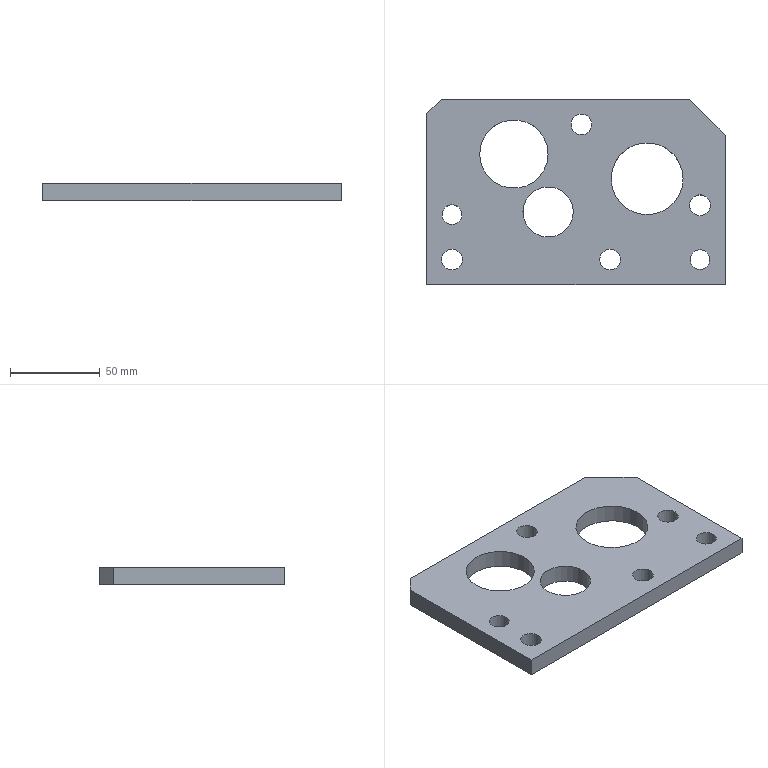Part | STEP file | lll_id4270_x_t | 1 solid | 17 faces | box 166 x 103.25 x 10 mm | volume 132948 mm3 | cylinder 9 | plane 8 | commonest cylinder face diameters 11.509 x4 11 x2 28 x1 38 x1 40 x1
STEP:
#1=CARTESIAN_POINT('',(3399.5,-57.,-45.));
#2=VERTEX_POINT('',#1);
#3=CARTESIAN_POINT('',(3419.5,-57.,-45.));
#4=DIRECTION('',(0.,0.,1.));
#5=DIRECTION('',(-1.,0.,0.));
#6=AXIS2_PLACEMENT_3D('',#3,#4,#5);
#7=CIRCLE('',#6,20.);
#8=EDGE_CURVE('',#2,#2,#7,.T.);
#9=ORIENTED_EDGE('',*,*,#8,.T.);
#10=EDGE_LOOP('',(#9));
#11=FACE_BOUND('',#10,.T.);
#12=CARTESIAN_POINT('',(3443.435,-102.,-45.));
#13=VERTEX_POINT('',#12);
#14=CARTESIAN_POINT('',(3448.935,-102.,-45.));
#15=DIRECTION('',(0.,0.,1.));
#16=DIRECTION('',(-1.,0.,0.));
#17=AXIS2_PLACEMENT_3D('',#14,#15,#16);
#18=CIRCLE('',#17,5.5);
#19=EDGE_CURVE('',#13,#13,#18,.T.);
#20=ORIENTED_EDGE('',*,*,#19,.T.);
#21=EDGE_LOOP('',(#20));
#22=FACE_BOUND('',#21,.T.);
#23=CARTESIAN_POINT('',(3304.935,-12.75,-45.));
#24=VERTEX_POINT('',#23);
#25=CARTESIAN_POINT('',(3442.935,-12.75,-45.));
#26=VERTEX_POINT('',#25);
#27=CARTESIAN_POINT('',(3580.234,-12.75,-45.));
#28=DIRECTION('',(1.,0.,0.));
#29=VECTOR('',#28,1.);
#30=LINE('',#27,#29);
#31=EDGE_CURVE('',#24,#26,#30,.T.);
#32=ORIENTED_EDGE('',*,*,#31,.T.);
#33=CARTESIAN_POINT('',(3462.935,-32.75,-45.));
#34=VERTEX_POINT('',#33);
#35=CARTESIAN_POINT('',(3455.935,-25.75,-45.));
#36=DIRECTION('',(-0.7071,0.7071,0.));
#37=VECTOR('',#36,1.);
#38=LINE('',#35,#37);
#39=EDGE_CURVE('',#34,#26,#38,.T.);
#40=ORIENTED_EDGE('',*,*,#39,.F.);
#41=CARTESIAN_POINT('',(3462.935,-116.,-45.));
#42=VERTEX_POINT('',#41);
#43=CARTESIAN_POINT('',(3462.935,-198.7,-45.));
#44=DIRECTION('',(0.,-1.,0.));
#45=VECTOR('',#44,1.);
#46=LINE('',#43,#45);
#47=EDGE_CURVE('',#34,#42,#46,.T.);
#48=ORIENTED_EDGE('',*,*,#47,.T.);
#49=CARTESIAN_POINT('',(3296.935,-116.,-45.));
#50=VERTEX_POINT('',#49);
#51=CARTESIAN_POINT('',(3580.234,-116.,-45.));
#52=DIRECTION('',(-1.,0.,0.));
#53=VECTOR('',#52,1.);
#54=LINE('',#51,#53);
#55=EDGE_CURVE('',#42,#50,#54,.T.);
#56=ORIENTED_EDGE('',*,*,#55,.T.);
#57=CARTESIAN_POINT('',(3296.935,-20.75,-45.));
#58=VERTEX_POINT('',#57);
#59=CARTESIAN_POINT('',(3296.935,-198.7,-45.));
#60=DIRECTION('',(0.,1.,0.));
#61=VECTOR('',#60,1.);
#62=LINE('',#59,#61);
#63=EDGE_CURVE('',#50,#58,#62,.T.);
#64=ORIENTED_EDGE('',*,*,#63,.T.);
#65=CARTESIAN_POINT('',(3179.435,-138.25,-45.));
#66=DIRECTION('',(-0.7071,-0.7071,0.));
#67=VECTOR('',#66,1.);
#68=LINE('',#65,#67);
#69=EDGE_CURVE('',#24,#58,#68,.T.);
#70=ORIENTED_EDGE('',*,*,#69,.F.);
#71=EDGE_LOOP('',(#32,#40,#48,#56,#64,#70));
#72=FACE_BOUND('',#71,.T.);
#73=CARTESIAN_POINT('',(3305.181,-102.,-45.));
#74=VERTEX_POINT('',#73);
#75=CARTESIAN_POINT('',(3310.935,-102.,-45.));
#76=DIRECTION('',(0.,0.,1.));
#77=DIRECTION('',(-1.,0.,0.));
#78=AXIS2_PLACEMENT_3D('',#75,#76,#77);
#79=CIRCLE('',#78,5.755);
#80=EDGE_CURVE('',#74,#74,#79,.T.);
#81=ORIENTED_EDGE('',*,*,#80,.T.);
#82=EDGE_LOOP('',(#81));
#83=FACE_BOUND('',#82,.T.);
#84=CARTESIAN_POINT('',(3305.435,-77.,-45.));
#85=VERTEX_POINT('',#84);
#86=CARTESIAN_POINT('',(3310.935,-77.,-45.));
#87=DIRECTION('',(0.,0.,1.));
#88=DIRECTION('',(-1.,0.,0.));
#89=AXIS2_PLACEMENT_3D('',#86,#87,#88);
#90=CIRCLE('',#89,5.5);
#91=EDGE_CURVE('',#85,#85,#90,.T.);
#92=ORIENTED_EDGE('',*,*,#91,.T.);
#93=EDGE_LOOP('',(#92));
#94=FACE_BOUND('',#93,.T.);
#95=CARTESIAN_POINT('',(3377.181,-26.75,-45.));
#96=VERTEX_POINT('',#95);
#97=CARTESIAN_POINT('',(3382.935,-26.75,-45.));
#98=DIRECTION('',(0.,0.,1.));
#99=DIRECTION('',(-1.,0.,0.));
#100=AXIS2_PLACEMENT_3D('',#97,#98,#99);
#101=CIRCLE('',#100,5.755);
#102=EDGE_CURVE('',#96,#96,#101,.T.);
#103=ORIENTED_EDGE('',*,*,#102,.T.);
#104=EDGE_LOOP('',(#103));
#105=FACE_BOUND('',#104,.T.);
#106=CARTESIAN_POINT('',(3393.181,-102.,-45.));
#107=VERTEX_POINT('',#106);
#108=CARTESIAN_POINT('',(3398.935,-102.,-45.));
#109=DIRECTION('',(0.,0.,1.));
#110=DIRECTION('',(-1.,0.,0.));
#111=AXIS2_PLACEMENT_3D('',#108,#109,#110);
#112=CIRCLE('',#111,5.755);
#113=EDGE_CURVE('',#107,#107,#112,.T.);
#114=ORIENTED_EDGE('',*,*,#113,.T.);
#115=EDGE_LOOP('',(#114));
#116=FACE_BOUND('',#115,.T.);
#117=CARTESIAN_POINT('',(3443.181,-71.75,-45.));
#118=VERTEX_POINT('',#117);
#119=CARTESIAN_POINT('',(3448.935,-71.75,-45.));
#120=DIRECTION('',(0.,0.,1.));
#121=DIRECTION('',(-1.,0.,0.));
#122=AXIS2_PLACEMENT_3D('',#119,#120,#121);
#123=CIRCLE('',#122,5.755);
#124=EDGE_CURVE('',#118,#118,#123,.T.);
#125=ORIENTED_EDGE('',*,*,#124,.T.);
#126=EDGE_LOOP('',(#125));
#127=FACE_BOUND('',#126,.T.);
#128=CARTESIAN_POINT('',(3350.435,-75.5,-45.));
#129=VERTEX_POINT('',#128);
#130=CARTESIAN_POINT('',(3364.435,-75.5,-45.));
#131=DIRECTION('',(0.,0.,-1.));
#132=DIRECTION('',(-1.,0.,0.));
#133=AXIS2_PLACEMENT_3D('',#130,#131,#132);
#134=CIRCLE('',#133,14.);
#135=EDGE_CURVE('',#129,#129,#134,.T.);
#136=ORIENTED_EDGE('',*,*,#135,.F.);
#137=EDGE_LOOP('',(#136));
#138=FACE_BOUND('',#137,.T.);
#139=CARTESIAN_POINT('',(3326.367,-43.288,-45.));
#140=VERTEX_POINT('',#139);
#141=CARTESIAN_POINT('',(3345.367,-43.288,-45.));
#142=DIRECTION('',(0.,0.,1.));
#143=DIRECTION('',(-1.,0.,0.));
#144=AXIS2_PLACEMENT_3D('',#141,#142,#143);
#145=CIRCLE('',#144,19.);
#146=EDGE_CURVE('',#140,#140,#145,.T.);
#147=ORIENTED_EDGE('',*,*,#146,.T.);
#148=EDGE_LOOP('',(#147));
#149=FACE_BOUND('',#148,.T.);
#150=CARTESIAN_POINT('',(3580.234,-198.7,-45.));
#151=DIRECTION('',(0.,0.,-1.));
#152=DIRECTION('',(0.,-1.,0.));
#153=AXIS2_PLACEMENT_3D('',#150,#151,#152);
#154=PLANE('',#153);
#155=ADVANCED_FACE('',(#11,#22,#72,#83,#94,#105,#116,#127,#138,#149),#154,.T.);
#156=CARTESIAN_POINT('',(3399.5,-57.,-35.));
#157=VERTEX_POINT('',#156);
#158=CARTESIAN_POINT('',(3419.5,-57.,-35.));
#159=DIRECTION('',(0.,0.,1.));
#160=DIRECTION('',(-1.,0.,0.));
#161=AXIS2_PLACEMENT_3D('',#158,#159,#160);
#162=CIRCLE('',#161,20.);
#163=EDGE_CURVE('',#157,#157,#162,.T.);
#164=ORIENTED_EDGE('',*,*,#163,.F.);
#165=EDGE_LOOP('',(#164));
#166=FACE_BOUND('',#165,.T.);
#167=CARTESIAN_POINT('',(3443.435,-102.,-35.));
#168=VERTEX_POINT('',#167);
#169=CARTESIAN_POINT('',(3448.935,-102.,-35.));
#170=DIRECTION('',(0.,0.,1.));
#171=DIRECTION('',(-1.,0.,0.));
#172=AXIS2_PLACEMENT_3D('',#169,#170,#171);
#173=CIRCLE('',#172,5.5);
#174=EDGE_CURVE('',#168,#168,#173,.T.);
#175=ORIENTED_EDGE('',*,*,#174,.F.);
#176=EDGE_LOOP('',(#175));
#177=FACE_BOUND('',#176,.T.);
#178=CARTESIAN_POINT('',(3304.935,-12.75,-35.));
#179=VERTEX_POINT('',#178);
#180=CARTESIAN_POINT('',(3442.935,-12.75,-35.));
#181=VERTEX_POINT('',#180);
#182=CARTESIAN_POINT('',(3266.435,-12.75,-35.));
#183=DIRECTION('',(1.,0.,0.));
#184=VECTOR('',#183,1.);
#185=LINE('',#182,#184);
#186=EDGE_CURVE('',#179,#181,#185,.T.);
#187=ORIENTED_EDGE('',*,*,#186,.F.);
#188=CARTESIAN_POINT('',(3296.935,-20.75,-35.));
#189=VERTEX_POINT('',#188);
#190=CARTESIAN_POINT('',(3179.435,-138.25,-35.));
#191=DIRECTION('',(-0.7071,-0.7071,0.));
#192=VECTOR('',#191,1.);
#193=LINE('',#190,#192);
#194=EDGE_CURVE('',#179,#189,#193,.T.);
#195=ORIENTED_EDGE('',*,*,#194,.T.);
#196=CARTESIAN_POINT('',(3296.935,-116.,-35.));
#197=VERTEX_POINT('',#196);
#198=CARTESIAN_POINT('',(3296.935,-215.25,-35.));
#199=DIRECTION('',(0.,1.,0.));
#200=VECTOR('',#199,1.);
#201=LINE('',#198,#200);
#202=EDGE_CURVE('',#197,#189,#201,.T.);
#203=ORIENTED_EDGE('',*,*,#202,.F.);
#204=CARTESIAN_POINT('',(3462.935,-116.,-35.));
#205=VERTEX_POINT('',#204);
#206=CARTESIAN_POINT('',(3266.435,-116.,-35.));
#207=DIRECTION('',(-1.,0.,0.));
#208=VECTOR('',#207,1.);
#209=LINE('',#206,#208);
#210=EDGE_CURVE('',#205,#197,#209,.T.);
#211=ORIENTED_EDGE('',*,*,#210,.F.);
#212=CARTESIAN_POINT('',(3462.935,-32.75,-35.));
#213=VERTEX_POINT('',#212);
#214=CARTESIAN_POINT('',(3462.935,-215.25,-35.));
#215=DIRECTION('',(0.,-1.,0.));
#216=VECTOR('',#215,1.);
#217=LINE('',#214,#216);
#218=EDGE_CURVE('',#213,#205,#217,.T.);
#219=ORIENTED_EDGE('',*,*,#218,.F.);
#220=CARTESIAN_POINT('',(3455.935,-25.75,-35.));
#221=DIRECTION('',(-0.7071,0.7071,0.));
#222=VECTOR('',#221,1.);
#223=LINE('',#220,#222);
#224=EDGE_CURVE('',#213,#181,#223,.T.);
#225=ORIENTED_EDGE('',*,*,#224,.T.);
#226=EDGE_LOOP('',(#187,#195,#203,#211,#219,#225));
#227=FACE_BOUND('',#226,.T.);
#228=CARTESIAN_POINT('',(3305.181,-102.,-35.));
#229=VERTEX_POINT('',#228);
#230=CARTESIAN_POINT('',(3310.935,-102.,-35.));
#231=DIRECTION('',(0.,0.,1.));
#232=DIRECTION('',(-1.,0.,0.));
#233=AXIS2_PLACEMENT_3D('',#230,#231,#232);
#234=CIRCLE('',#233,5.755);
#235=EDGE_CURVE('',#229,#229,#234,.T.);
#236=ORIENTED_EDGE('',*,*,#235,.F.);
#237=EDGE_LOOP('',(#236));
#238=FACE_BOUND('',#237,.T.);
#239=CARTESIAN_POINT('',(3305.435,-77.,-35.));
#240=VERTEX_POINT('',#239);
#241=CARTESIAN_POINT('',(3310.935,-77.,-35.));
#242=DIRECTION('',(0.,0.,1.));
#243=DIRECTION('',(-1.,0.,0.));
#244=AXIS2_PLACEMENT_3D('',#241,#242,#243);
#245=CIRCLE('',#244,5.5);
#246=EDGE_CURVE('',#240,#240,#245,.T.);
#247=ORIENTED_EDGE('',*,*,#246,.F.);
#248=EDGE_LOOP('',(#247));
#249=FACE_BOUND('',#248,.T.);
#250=CARTESIAN_POINT('',(3377.181,-26.75,-35.));
#251=VERTEX_POINT('',#250);
#252=CARTESIAN_POINT('',(3382.935,-26.75,-35.));
#253=DIRECTION('',(0.,0.,1.));
#254=DIRECTION('',(-1.,0.,0.));
#255=AXIS2_PLACEMENT_3D('',#252,#253,#254);
#256=CIRCLE('',#255,5.755);
#257=EDGE_CURVE('',#251,#251,#256,.T.);
#258=ORIENTED_EDGE('',*,*,#257,.F.);
#259=EDGE_LOOP('',(#258));
#260=FACE_BOUND('',#259,.T.);
#261=CARTESIAN_POINT('',(3393.181,-102.,-35.));
#262=VERTEX_POINT('',#261);
#263=CARTESIAN_POINT('',(3398.935,-102.,-35.));
#264=DIRECTION('',(0.,0.,1.));
#265=DIRECTION('',(-1.,0.,0.));
#266=AXIS2_PLACEMENT_3D('',#263,#264,#265);
#267=CIRCLE('',#266,5.755);
#268=EDGE_CURVE('',#262,#262,#267,.T.);
#269=ORIENTED_EDGE('',*,*,#268,.F.);
#270=EDGE_LOOP('',(#269));
#271=FACE_BOUND('',#270,.T.);
#272=CARTESIAN_POINT('',(3443.181,-71.75,-35.));
#273=VERTEX_POINT('',#272);
#274=CARTESIAN_POINT('',(3448.935,-71.75,-35.));
#275=DIRECTION('',(0.,0.,1.));
#276=DIRECTION('',(-1.,0.,0.));
#277=AXIS2_PLACEMENT_3D('',#274,#275,#276);
#278=CIRCLE('',#277,5.755);
#279=EDGE_CURVE('',#273,#273,#278,.T.);
#280=ORIENTED_EDGE('',*,*,#279,.F.);
#281=EDGE_LOOP('',(#280));
#282=FACE_BOUND('',#281,.T.);
#283=CARTESIAN_POINT('',(3350.435,-75.5,-35.));
#284=VERTEX_POINT('',#283);
#285=CARTESIAN_POINT('',(3364.435,-75.5,-35.));
#286=DIRECTION('',(0.,0.,-1.));
#287=DIRECTION('',(-1.,0.,0.));
#288=AXIS2_PLACEMENT_3D('',#285,#286,#287);
#289=CIRCLE('',#288,14.);
#290=EDGE_CURVE('',#284,#284,#289,.T.);
#291=ORIENTED_EDGE('',*,*,#290,.T.);
#292=EDGE_LOOP('',(#291));
#293=FACE_BOUND('',#292,.T.);
#294=CARTESIAN_POINT('',(3326.367,-43.288,-35.));
#295=VERTEX_POINT('',#294);
#296=CARTESIAN_POINT('',(3345.367,-43.288,-35.));
#297=DIRECTION('',(0.,0.,1.));
#298=DIRECTION('',(-1.,0.,0.));
#299=AXIS2_PLACEMENT_3D('',#296,#297,#298);
#300=CIRCLE('',#299,19.);
#301=EDGE_CURVE('',#295,#295,#300,.T.);
#302=ORIENTED_EDGE('',*,*,#301,.F.);
#303=EDGE_LOOP('',(#302));
#304=FACE_BOUND('',#303,.T.);
#305=CARTESIAN_POINT('',(3266.435,-215.25,-35.));
#306=DIRECTION('',(0.,0.,-1.));
#307=DIRECTION('',(1.,0.,0.));
#308=AXIS2_PLACEMENT_3D('',#305,#306,#307);
#309=PLANE('',#308);
#310=ADVANCED_FACE('',(#166,#177,#227,#238,#249,#260,#271,#282,#293,#304),#309,.F.);
#311=CARTESIAN_POINT('',(3462.935,-32.75,-35.));
#312=DIRECTION('',(0.,0.,-1.));
#313=VECTOR('',#312,1.);
#314=LINE('',#311,#313);
#315=EDGE_CURVE('',#213,#34,#314,.T.);
#316=ORIENTED_EDGE('',*,*,#315,.F.);
#317=ORIENTED_EDGE('',*,*,#218,.T.);
#318=CARTESIAN_POINT('',(3462.935,-116.,-35.));
#319=DIRECTION('',(0.,0.,-1.));
#320=VECTOR('',#319,1.);
#321=LINE('',#318,#320);
#322=EDGE_CURVE('',#205,#42,#321,.T.);
#323=ORIENTED_EDGE('',*,*,#322,.T.);
#324=ORIENTED_EDGE('',*,*,#47,.F.);
#325=EDGE_LOOP('',(#316,#317,#323,#324));
#326=FACE_OUTER_BOUND('',#325,.T.);
#327=CARTESIAN_POINT('',(3462.935,-215.25,-35.));
#328=DIRECTION('',(1.,0.,0.));
#329=DIRECTION('',(0.,-1.,0.));
#330=AXIS2_PLACEMENT_3D('',#327,#328,#329);
#331=PLANE('',#330);
#332=ADVANCED_FACE('',(#326),#331,.T.);
#333=ORIENTED_EDGE('',*,*,#322,.F.);
#334=ORIENTED_EDGE('',*,*,#210,.T.);
#335=CARTESIAN_POINT('',(3296.935,-116.,-35.));
#336=DIRECTION('',(0.,0.,-1.));
#337=VECTOR('',#336,1.);
#338=LINE('',#335,#337);
#339=EDGE_CURVE('',#197,#50,#338,.T.);
#340=ORIENTED_EDGE('',*,*,#339,.T.);
#341=ORIENTED_EDGE('',*,*,#55,.F.);
#342=EDGE_LOOP('',(#333,#334,#340,#341));
#343=FACE_OUTER_BOUND('',#342,.T.);
#344=CARTESIAN_POINT('',(3266.435,-116.,-35.));
#345=DIRECTION('',(0.,-1.,0.));
#346=DIRECTION('',(-1.,0.,0.));
#347=AXIS2_PLACEMENT_3D('',#344,#345,#346);
#348=PLANE('',#347);
#349=ADVANCED_FACE('',(#343),#348,.T.);
#350=ORIENTED_EDGE('',*,*,#339,.F.);
#351=ORIENTED_EDGE('',*,*,#202,.T.);
#352=CARTESIAN_POINT('',(3296.935,-20.75,-35.));
#353=DIRECTION('',(0.,0.,-1.));
#354=VECTOR('',#353,1.);
#355=LINE('',#352,#354);
#356=EDGE_CURVE('',#189,#58,#355,.T.);
#357=ORIENTED_EDGE('',*,*,#356,.T.);
#358=ORIENTED_EDGE('',*,*,#63,.F.);
#359=EDGE_LOOP('',(#350,#351,#357,#358));
#360=FACE_OUTER_BOUND('',#359,.T.);
#361=CARTESIAN_POINT('',(3296.935,-215.25,-35.));
#362=DIRECTION('',(-1.,0.,0.));
#363=DIRECTION('',(0.,1.,0.));
#364=AXIS2_PLACEMENT_3D('',#361,#362,#363);
#365=PLANE('',#364);
#366=ADVANCED_FACE('',(#360),#365,.T.);
#367=ORIENTED_EDGE('',*,*,#356,.F.);
#368=ORIENTED_EDGE('',*,*,#194,.F.);
#369=CARTESIAN_POINT('',(3304.935,-12.75,-35.));
#370=DIRECTION('',(0.,0.,-1.));
#371=VECTOR('',#370,1.);
#372=LINE('',#369,#371);
#373=EDGE_CURVE('',#179,#24,#372,.T.);
#374=ORIENTED_EDGE('',*,*,#373,.T.);
#375=ORIENTED_EDGE('',*,*,#69,.T.);
#376=EDGE_LOOP('',(#367,#368,#374,#375));
#377=FACE_OUTER_BOUND('',#376,.T.);
#378=CARTESIAN_POINT('',(3179.435,-138.25,-35.));
#379=DIRECTION('',(0.7071,-0.7071,0.));
#380=DIRECTION('',(-0.7071,-0.7071,0.));
#381=AXIS2_PLACEMENT_3D('',#378,#379,#380);
#382=PLANE('',#381);
#383=ADVANCED_FACE('',(#377),#382,.F.);
#384=ORIENTED_EDGE('',*,*,#373,.F.);
#385=ORIENTED_EDGE('',*,*,#186,.T.);
#386=CARTESIAN_POINT('',(3442.935,-12.75,-35.));
#387=DIRECTION('',(0.,0.,-1.));
#388=VECTOR('',#387,1.);
#389=LINE('',#386,#388);
#390=EDGE_CURVE('',#181,#26,#389,.T.);
#391=ORIENTED_EDGE('',*,*,#390,.T.);
#392=ORIENTED_EDGE('',*,*,#31,.F.);
#393=EDGE_LOOP('',(#384,#385,#391,#392));
#394=FACE_OUTER_BOUND('',#393,.T.);
#395=CARTESIAN_POINT('',(3266.435,-12.75,-35.));
#396=DIRECTION('',(0.,1.,0.));
#397=DIRECTION('',(1.,0.,0.));
#398=AXIS2_PLACEMENT_3D('',#395,#396,#397);
#399=PLANE('',#398);
#400=ADVANCED_FACE('',(#394),#399,.T.);
#401=ORIENTED_EDGE('',*,*,#124,.F.);
#402=EDGE_LOOP('',(#401));
#403=FACE_BOUND('',#402,.T.);
#404=ORIENTED_EDGE('',*,*,#279,.T.);
#405=EDGE_LOOP('',(#404));
#406=FACE_BOUND('',#405,.T.);
#407=CARTESIAN_POINT('',(3448.935,-71.75,-35.));
#408=DIRECTION('',(0.,0.,1.));
#409=DIRECTION('',(1.,0.,0.));
#410=AXIS2_PLACEMENT_3D('',#407,#408,#409);
#411=CYLINDRICAL_SURFACE('',#410,5.755);
#412=ADVANCED_FACE('',(#403,#406),#411,.F.);
#413=ORIENTED_EDGE('',*,*,#113,.F.);
#414=EDGE_LOOP('',(#413));
#415=FACE_BOUND('',#414,.T.);
#416=ORIENTED_EDGE('',*,*,#268,.T.);
#417=EDGE_LOOP('',(#416));
#418=FACE_BOUND('',#417,.T.);
#419=CARTESIAN_POINT('',(3398.935,-102.,-35.));
#420=DIRECTION('',(0.,0.,1.));
#421=DIRECTION('',(1.,0.,0.));
#422=AXIS2_PLACEMENT_3D('',#419,#420,#421);
#423=CYLINDRICAL_SURFACE('',#422,5.755);
#424=ADVANCED_FACE('',(#415,#418),#423,.F.);
#425=ORIENTED_EDGE('',*,*,#102,.F.);
#426=EDGE_LOOP('',(#425));
#427=FACE_BOUND('',#426,.T.);
#428=ORIENTED_EDGE('',*,*,#257,.T.);
#429=EDGE_LOOP('',(#428));
#430=FACE_BOUND('',#429,.T.);
#431=CARTESIAN_POINT('',(3382.935,-26.75,-35.));
#432=DIRECTION('',(0.,0.,1.));
#433=DIRECTION('',(1.,0.,0.));
#434=AXIS2_PLACEMENT_3D('',#431,#432,#433);
#435=CYLINDRICAL_SURFACE('',#434,5.755);
#436=ADVANCED_FACE('',(#427,#430),#435,.F.);
#437=ORIENTED_EDGE('',*,*,#91,.F.);
#438=EDGE_LOOP('',(#437));
#439=FACE_BOUND('',#438,.T.);
#440=ORIENTED_EDGE('',*,*,#246,.T.);
#441=EDGE_LOOP('',(#440));
#442=FACE_BOUND('',#441,.T.);
#443=CARTESIAN_POINT('',(3310.935,-77.,-35.));
#444=DIRECTION('',(0.,0.,1.));
#445=DIRECTION('',(1.,0.,0.));
#446=AXIS2_PLACEMENT_3D('',#443,#444,#445);
#447=CYLINDRICAL_SURFACE('',#446,5.5);
#448=ADVANCED_FACE('',(#439,#442),#447,.F.);
#449=ORIENTED_EDGE('',*,*,#80,.F.);
#450=EDGE_LOOP('',(#449));
#451=FACE_BOUND('',#450,.T.);
#452=ORIENTED_EDGE('',*,*,#235,.T.);
#453=EDGE_LOOP('',(#452));
#454=FACE_BOUND('',#453,.T.);
#455=CARTESIAN_POINT('',(3310.935,-102.,-35.));
#456=DIRECTION('',(0.,0.,1.));
#457=DIRECTION('',(1.,0.,0.));
#458=AXIS2_PLACEMENT_3D('',#455,#456,#457);
#459=CYLINDRICAL_SURFACE('',#458,5.755);
#460=ADVANCED_FACE('',(#451,#454),#459,.F.);
#461=ORIENTED_EDGE('',*,*,#224,.F.);
#462=ORIENTED_EDGE('',*,*,#315,.T.);
#463=ORIENTED_EDGE('',*,*,#39,.T.);
#464=ORIENTED_EDGE('',*,*,#390,.F.);
#465=EDGE_LOOP('',(#461,#462,#463,#464));
#466=FACE_OUTER_BOUND('',#465,.T.);
#467=CARTESIAN_POINT('',(3455.935,-25.75,-35.));
#468=DIRECTION('',(0.7071,0.7071,0.));
#469=DIRECTION('',(0.7071,-0.7071,0.));
#470=AXIS2_PLACEMENT_3D('',#467,#468,#469);
#471=PLANE('',#470);
#472=ADVANCED_FACE('',(#466),#471,.T.);
#473=ORIENTED_EDGE('',*,*,#19,.F.);
#474=EDGE_LOOP('',(#473));
#475=FACE_BOUND('',#474,.T.);
#476=ORIENTED_EDGE('',*,*,#174,.T.);
#477=EDGE_LOOP('',(#476));
#478=FACE_BOUND('',#477,.T.);
#479=CARTESIAN_POINT('',(3448.935,-102.,-35.));
#480=DIRECTION('',(0.,0.,1.));
#481=DIRECTION('',(1.,0.,0.));
#482=AXIS2_PLACEMENT_3D('',#479,#480,#481);
#483=CYLINDRICAL_SURFACE('',#482,5.5);
#484=ADVANCED_FACE('',(#475,#478),#483,.F.);
#485=ORIENTED_EDGE('',*,*,#8,.F.);
#486=EDGE_LOOP('',(#485));
#487=FACE_BOUND('',#486,.T.);
#488=ORIENTED_EDGE('',*,*,#163,.T.);
#489=EDGE_LOOP('',(#488));
#490=FACE_BOUND('',#489,.T.);
#491=CARTESIAN_POINT('',(3419.5,-57.,-35.));
#492=DIRECTION('',(0.,0.,-1.));
#493=DIRECTION('',(-1.,0.,0.));
#494=AXIS2_PLACEMENT_3D('',#491,#492,#493);
#495=CYLINDRICAL_SURFACE('',#494,20.);
#496=ADVANCED_FACE('',(#487,#490),#495,.F.);
#497=ORIENTED_EDGE('',*,*,#135,.T.);
#498=EDGE_LOOP('',(#497));
#499=FACE_BOUND('',#498,.T.);
#500=ORIENTED_EDGE('',*,*,#290,.F.);
#501=EDGE_LOOP('',(#500));
#502=FACE_BOUND('',#501,.T.);
#503=CARTESIAN_POINT('',(3364.435,-75.5,-235.));
#504=DIRECTION('',(0.,0.,1.));
#505=DIRECTION('',(1.,0.,0.));
#506=AXIS2_PLACEMENT_3D('',#503,#504,#505);
#507=CYLINDRICAL_SURFACE('',#506,14.);
#508=ADVANCED_FACE('',(#499,#502),#507,.F.);
#509=ORIENTED_EDGE('',*,*,#146,.F.);
#510=EDGE_LOOP('',(#509));
#511=FACE_BOUND('',#510,.T.);
#512=ORIENTED_EDGE('',*,*,#301,.T.);
#513=EDGE_LOOP('',(#512));
#514=FACE_BOUND('',#513,.T.);
#515=CARTESIAN_POINT('',(3345.367,-43.288,-235.));
#516=DIRECTION('',(0.,0.,1.));
#517=DIRECTION('',(1.,0.,0.));
#518=AXIS2_PLACEMENT_3D('',#515,#516,#517);
#519=CYLINDRICAL_SURFACE('',#518,19.);
#520=ADVANCED_FACE('',(#511,#514),#519,.F.);
#521=CLOSED_SHELL('',(#155,#310,#332,#349,#366,#383,#400,#412,#424,#436,#448,#460,#472,#484,#496,#508,#520));
#522=MANIFOLD_SOLID_BREP('',#521);
#523=(LENGTH_UNIT()NAMED_UNIT(*)SI_UNIT(.MILLI.,.METRE.));
#524=UNCERTAINTY_MEASURE_WITH_UNIT(LENGTH_MEASURE(0.00002),#523,'','');
#525=(NAMED_UNIT(*)PLANE_ANGLE_UNIT()SI_UNIT($,.RADIAN.));
#526=PLANE_ANGLE_MEASURE_WITH_UNIT(PLANE_ANGLE_MEASURE(0.01745),#525);
#527=DIMENSIONAL_EXPONENTS(0.,0.,0.,0.,0.,0.,0.);
#528=(CONVERSION_BASED_UNIT('DEGREE',#526)NAMED_UNIT(#527)PLANE_ANGLE_UNIT());
#529=(NAMED_UNIT(*)SI_UNIT($,.STERADIAN.)SOLID_ANGLE_UNIT());
#530=(GEOMETRIC_REPRESENTATION_CONTEXT(3)GLOBAL_UNCERTAINTY_ASSIGNED_CONTEXT((#524))GLOBAL_UNIT_ASSIGNED_CONTEXT((#523,#528,#529))REPRESENTATION_CONTEXT('',''));
#531=ADVANCED_BREP_SHAPE_REPRESENTATION('',(#522),#530);